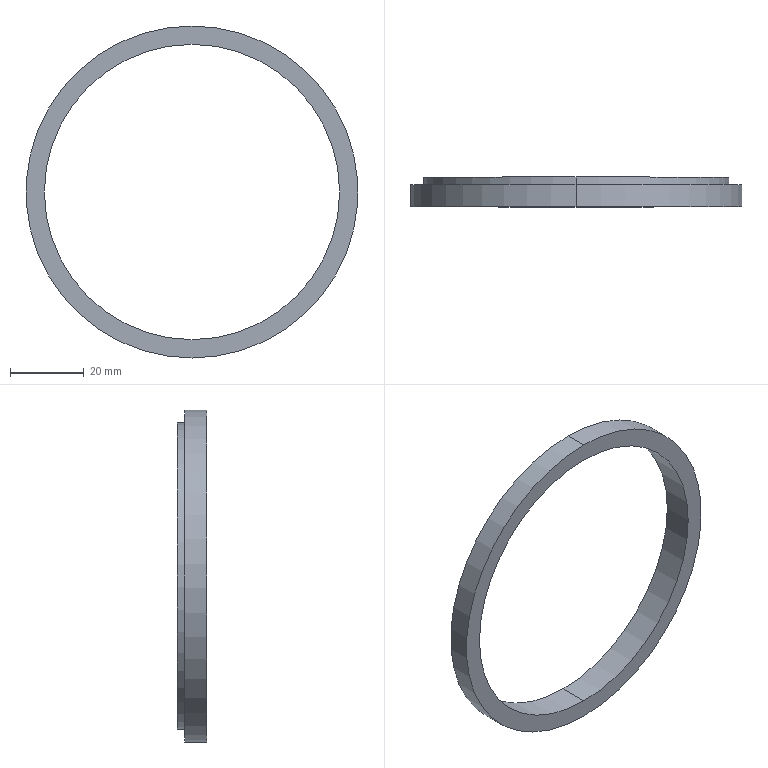Part | SolidWorks | features Extrusion 1, ICE 1 | 1 solid | 9 faces | box 90 x 8 x 90 mm | volume 8779 mm3 | cylinder 6 | plane 3 | commonest cylinder face diameters 80 x2 83 x2 90 x2
STEP:
#1=CARTESIAN_POINT('',(0.,8.,41.5));
#2=VERTEX_POINT('',#1);
#3=CARTESIAN_POINT('',(0.,8.,-41.5));
#4=VERTEX_POINT('',#3);
#5=CARTESIAN_POINT('',(0.,8.,0.));
#6=DIRECTION('',(0.,1.,0.));
#7=DIRECTION('',(0.,0.,1.));
#8=AXIS2_PLACEMENT_3D('',#5,#6,#7);
#9=CIRCLE('',#8,41.5);
#10=EDGE_CURVE('',#2,#4,#9,.T.);
#11=ORIENTED_EDGE('',*,*,#10,.F.);
#12=CARTESIAN_POINT('',(0.,6.,41.5));
#13=VERTEX_POINT('',#12);
#14=CARTESIAN_POINT('',(0.,8.,41.5));
#15=DIRECTION('',(0.,-1.,0.));
#16=VECTOR('',#15,1000.);
#17=LINE('',#14,#16);
#18=EDGE_CURVE('',#2,#13,#17,.T.);
#19=ORIENTED_EDGE('',*,*,#18,.T.);
#20=CARTESIAN_POINT('',(0.,6.,-41.5));
#21=VERTEX_POINT('',#20);
#22=CARTESIAN_POINT('',(0.,6.,0.));
#23=DIRECTION('',(0.,1.,0.));
#24=DIRECTION('',(0.,0.,1.));
#25=AXIS2_PLACEMENT_3D('',#22,#23,#24);
#26=CIRCLE('',#25,41.5);
#27=EDGE_CURVE('',#13,#21,#26,.T.);
#28=ORIENTED_EDGE('',*,*,#27,.T.);
#29=CARTESIAN_POINT('',(0.,8.,-41.5));
#30=DIRECTION('',(0.,-1.,0.));
#31=VECTOR('',#30,1000.);
#32=LINE('',#29,#31);
#33=EDGE_CURVE('',#4,#21,#32,.T.);
#34=ORIENTED_EDGE('',*,*,#33,.F.);
#35=EDGE_LOOP('',(#11,#19,#28,#34));
#36=FACE_OUTER_BOUND('',#35,.T.);
#37=CARTESIAN_POINT('',(0.,8.,0.));
#38=DIRECTION('',(0.,-1.,0.));
#39=DIRECTION('',(0.,0.,-1.));
#40=AXIS2_PLACEMENT_3D('',#37,#38,#39);
#41=CYLINDRICAL_SURFACE('',#40,41.5);
#42=ADVANCED_FACE('',(#36),#41,.T.);
#43=CARTESIAN_POINT('',(0.,8.,-40.));
#44=VERTEX_POINT('',#43);
#45=CARTESIAN_POINT('',(0.,8.,40.));
#46=VERTEX_POINT('',#45);
#47=CARTESIAN_POINT('',(0.,8.,0.));
#48=DIRECTION('',(0.,1.,0.));
#49=DIRECTION('',(0.,0.,1.));
#50=AXIS2_PLACEMENT_3D('',#47,#48,#49);
#51=CIRCLE('',#50,40.);
#52=EDGE_CURVE('',#44,#46,#51,.T.);
#53=ORIENTED_EDGE('',*,*,#52,.T.);
#54=CARTESIAN_POINT('',(0.,0.,40.));
#55=VERTEX_POINT('',#54);
#56=CARTESIAN_POINT('',(0.,6.,40.));
#57=DIRECTION('',(0.,-1.,0.));
#58=VECTOR('',#57,1000.);
#59=LINE('',#56,#58);
#60=EDGE_CURVE('',#46,#55,#59,.T.);
#61=ORIENTED_EDGE('',*,*,#60,.T.);
#62=CARTESIAN_POINT('',(0.,0.,-40.));
#63=VERTEX_POINT('',#62);
#64=CARTESIAN_POINT('',(0.,0.,0.));
#65=DIRECTION('',(0.,1.,0.));
#66=DIRECTION('',(0.,0.,1.));
#67=AXIS2_PLACEMENT_3D('',#64,#65,#66);
#68=CIRCLE('',#67,40.);
#69=EDGE_CURVE('',#63,#55,#68,.T.);
#70=ORIENTED_EDGE('',*,*,#69,.F.);
#71=CARTESIAN_POINT('',(0.,6.,-40.));
#72=DIRECTION('',(0.,-1.,0.));
#73=VECTOR('',#72,1000.);
#74=LINE('',#71,#73);
#75=EDGE_CURVE('',#44,#63,#74,.T.);
#76=ORIENTED_EDGE('',*,*,#75,.F.);
#77=EDGE_LOOP('',(#53,#61,#70,#76));
#78=FACE_OUTER_BOUND('',#77,.T.);
#79=CARTESIAN_POINT('',(0.,6.,0.));
#80=DIRECTION('',(0.,-1.,0.));
#81=DIRECTION('',(0.,0.,-1.));
#82=AXIS2_PLACEMENT_3D('',#79,#80,#81);
#83=CYLINDRICAL_SURFACE('',#82,40.);
#84=ADVANCED_FACE('',(#78),#83,.F.);
#85=CARTESIAN_POINT('',(0.,6.,45.));
#86=VERTEX_POINT('',#85);
#87=CARTESIAN_POINT('',(0.,6.,-45.));
#88=VERTEX_POINT('',#87);
#89=CARTESIAN_POINT('',(0.,6.,0.));
#90=DIRECTION('',(0.,1.,0.));
#91=DIRECTION('',(0.,0.,1.));
#92=AXIS2_PLACEMENT_3D('',#89,#90,#91);
#93=CIRCLE('',#92,45.);
#94=EDGE_CURVE('',#86,#88,#93,.T.);
#95=ORIENTED_EDGE('',*,*,#94,.F.);
#96=CARTESIAN_POINT('',(0.,0.,45.));
#97=VERTEX_POINT('',#96);
#98=CARTESIAN_POINT('',(0.,6.,45.));
#99=DIRECTION('',(0.,-1.,0.));
#100=VECTOR('',#99,1000.);
#101=LINE('',#98,#100);
#102=EDGE_CURVE('',#86,#97,#101,.T.);
#103=ORIENTED_EDGE('',*,*,#102,.T.);
#104=CARTESIAN_POINT('',(0.,0.,-45.));
#105=VERTEX_POINT('',#104);
#106=CARTESIAN_POINT('',(0.,0.,0.));
#107=DIRECTION('',(0.,1.,0.));
#108=DIRECTION('',(0.,0.,1.));
#109=AXIS2_PLACEMENT_3D('',#106,#107,#108);
#110=CIRCLE('',#109,45.);
#111=EDGE_CURVE('',#97,#105,#110,.T.);
#112=ORIENTED_EDGE('',*,*,#111,.T.);
#113=CARTESIAN_POINT('',(0.,6.,-45.));
#114=DIRECTION('',(0.,-1.,0.));
#115=VECTOR('',#114,1000.);
#116=LINE('',#113,#115);
#117=EDGE_CURVE('',#88,#105,#116,.T.);
#118=ORIENTED_EDGE('',*,*,#117,.F.);
#119=EDGE_LOOP('',(#95,#103,#112,#118));
#120=FACE_OUTER_BOUND('',#119,.T.);
#121=CARTESIAN_POINT('',(0.,6.,0.));
#122=DIRECTION('',(0.,-1.,0.));
#123=DIRECTION('',(0.,0.,-1.));
#124=AXIS2_PLACEMENT_3D('',#121,#122,#123);
#125=CYLINDRICAL_SURFACE('',#124,45.);
#126=ADVANCED_FACE('',(#120),#125,.T.);
#127=CARTESIAN_POINT('',(0.,6.,0.));
#128=DIRECTION('',(0.,1.,0.));
#129=DIRECTION('',(0.,0.,1.));
#130=AXIS2_PLACEMENT_3D('',#127,#128,#129);
#131=CIRCLE('',#130,45.);
#132=EDGE_CURVE('',#88,#86,#131,.T.);
#133=ORIENTED_EDGE('',*,*,#132,.T.);
#134=ORIENTED_EDGE('',*,*,#94,.T.);
#135=EDGE_LOOP('',(#133,#134));
#136=FACE_OUTER_BOUND('',#135,.T.);
#137=CARTESIAN_POINT('',(0.,6.,0.));
#138=DIRECTION('',(0.,1.,0.));
#139=DIRECTION('',(0.,0.,1.));
#140=AXIS2_PLACEMENT_3D('',#137,#138,#139);
#141=CIRCLE('',#140,41.5);
#142=EDGE_CURVE('',#21,#13,#141,.T.);
#143=ORIENTED_EDGE('',*,*,#142,.F.);
#144=ORIENTED_EDGE('',*,*,#27,.F.);
#145=EDGE_LOOP('',(#143,#144));
#146=FACE_BOUND('',#145,.T.);
#147=CARTESIAN_POINT('',(0.,6.,0.));
#148=DIRECTION('',(0.,1.,0.));
#149=DIRECTION('',(0.,0.,1.));
#150=AXIS2_PLACEMENT_3D('',#147,#148,#149);
#151=PLANE('',#150);
#152=ADVANCED_FACE('',(#136,#146),#151,.T.);
#153=CARTESIAN_POINT('',(0.,0.,0.));
#154=DIRECTION('',(0.,1.,0.));
#155=DIRECTION('',(0.,0.,1.));
#156=AXIS2_PLACEMENT_3D('',#153,#154,#155);
#157=CIRCLE('',#156,45.);
#158=EDGE_CURVE('',#105,#97,#157,.T.);
#159=ORIENTED_EDGE('',*,*,#158,.F.);
#160=ORIENTED_EDGE('',*,*,#111,.F.);
#161=EDGE_LOOP('',(#159,#160));
#162=FACE_OUTER_BOUND('',#161,.T.);
#163=ORIENTED_EDGE('',*,*,#69,.T.);
#164=CARTESIAN_POINT('',(0.,0.,0.));
#165=DIRECTION('',(0.,1.,0.));
#166=DIRECTION('',(0.,0.,1.));
#167=AXIS2_PLACEMENT_3D('',#164,#165,#166);
#168=CIRCLE('',#167,40.);
#169=EDGE_CURVE('',#55,#63,#168,.T.);
#170=ORIENTED_EDGE('',*,*,#169,.T.);
#171=EDGE_LOOP('',(#163,#170));
#172=FACE_BOUND('',#171,.T.);
#173=CARTESIAN_POINT('',(0.,0.,0.));
#174=DIRECTION('',(0.,1.,0.));
#175=DIRECTION('',(0.,0.,1.));
#176=AXIS2_PLACEMENT_3D('',#173,#174,#175);
#177=PLANE('',#176);
#178=ADVANCED_FACE('',(#162,#172),#177,.F.);
#179=ORIENTED_EDGE('',*,*,#102,.F.);
#180=ORIENTED_EDGE('',*,*,#132,.F.);
#181=ORIENTED_EDGE('',*,*,#117,.T.);
#182=ORIENTED_EDGE('',*,*,#158,.T.);
#183=EDGE_LOOP('',(#179,#180,#181,#182));
#184=FACE_OUTER_BOUND('',#183,.T.);
#185=CARTESIAN_POINT('',(0.,6.,0.));
#186=DIRECTION('',(0.,-1.,0.));
#187=DIRECTION('',(0.,0.,-1.));
#188=AXIS2_PLACEMENT_3D('',#185,#186,#187);
#189=CYLINDRICAL_SURFACE('',#188,45.);
#190=ADVANCED_FACE('',(#184),#189,.T.);
#191=ORIENTED_EDGE('',*,*,#60,.F.);
#192=CARTESIAN_POINT('',(0.,8.,0.));
#193=DIRECTION('',(0.,1.,0.));
#194=DIRECTION('',(0.,0.,1.));
#195=AXIS2_PLACEMENT_3D('',#192,#193,#194);
#196=CIRCLE('',#195,40.);
#197=EDGE_CURVE('',#46,#44,#196,.T.);
#198=ORIENTED_EDGE('',*,*,#197,.T.);
#199=ORIENTED_EDGE('',*,*,#75,.T.);
#200=ORIENTED_EDGE('',*,*,#169,.F.);
#201=EDGE_LOOP('',(#191,#198,#199,#200));
#202=FACE_OUTER_BOUND('',#201,.T.);
#203=CARTESIAN_POINT('',(0.,6.,0.));
#204=DIRECTION('',(0.,-1.,0.));
#205=DIRECTION('',(0.,0.,-1.));
#206=AXIS2_PLACEMENT_3D('',#203,#204,#205);
#207=CYLINDRICAL_SURFACE('',#206,40.);
#208=ADVANCED_FACE('',(#202),#207,.F.);
#209=CARTESIAN_POINT('',(0.,8.,0.));
#210=DIRECTION('',(0.,1.,0.));
#211=DIRECTION('',(0.,0.,1.));
#212=AXIS2_PLACEMENT_3D('',#209,#210,#211);
#213=CIRCLE('',#212,41.5);
#214=EDGE_CURVE('',#4,#2,#213,.T.);
#215=ORIENTED_EDGE('',*,*,#214,.T.);
#216=ORIENTED_EDGE('',*,*,#10,.T.);
#217=EDGE_LOOP('',(#215,#216));
#218=FACE_OUTER_BOUND('',#217,.T.);
#219=ORIENTED_EDGE('',*,*,#52,.F.);
#220=ORIENTED_EDGE('',*,*,#197,.F.);
#221=EDGE_LOOP('',(#219,#220));
#222=FACE_BOUND('',#221,.T.);
#223=CARTESIAN_POINT('',(0.,8.,0.));
#224=DIRECTION('',(0.,1.,0.));
#225=DIRECTION('',(0.,0.,1.));
#226=AXIS2_PLACEMENT_3D('',#223,#224,#225);
#227=PLANE('',#226);
#228=ADVANCED_FACE('',(#218,#222),#227,.T.);
#229=ORIENTED_EDGE('',*,*,#18,.F.);
#230=ORIENTED_EDGE('',*,*,#214,.F.);
#231=ORIENTED_EDGE('',*,*,#33,.T.);
#232=ORIENTED_EDGE('',*,*,#142,.T.);
#233=EDGE_LOOP('',(#229,#230,#231,#232));
#234=FACE_OUTER_BOUND('',#233,.T.);
#235=CARTESIAN_POINT('',(0.,8.,0.));
#236=DIRECTION('',(0.,-1.,0.));
#237=DIRECTION('',(0.,0.,-1.));
#238=AXIS2_PLACEMENT_3D('',#235,#236,#237);
#239=CYLINDRICAL_SURFACE('',#238,41.5);
#240=ADVANCED_FACE('',(#234),#239,.T.);
#241=CLOSED_SHELL('',(#42,#84,#126,#152,#178,#190,#208,#228,#240));
#242=MANIFOLD_SOLID_BREP('',#241);
#243=CARTESIAN_POINT('',(0.,0.,0.));
#244=DIRECTION('',(0.,0.,1.));
#245=DIRECTION('',(1.,0.,0.));
#246=AXIS2_PLACEMENT_3D('',#243,#244,#245);
#247=(LENGTH_UNIT()NAMED_UNIT(*)SI_UNIT(.MILLI.,.METRE.));
#248=UNCERTAINTY_MEASURE_WITH_UNIT(LENGTH_MEASURE(0.00001),#247,'','');
#249=(NAMED_UNIT(*)PLANE_ANGLE_UNIT()SI_UNIT($,.RADIAN.));
#250=(NAMED_UNIT(*)SI_UNIT($,.STERADIAN.)SOLID_ANGLE_UNIT());
#251=(GEOMETRIC_REPRESENTATION_CONTEXT(3)GLOBAL_UNCERTAINTY_ASSIGNED_CONTEXT((#248))GLOBAL_UNIT_ASSIGNED_CONTEXT((#247,#249,#250))REPRESENTATION_CONTEXT('',''));
#252=ADVANCED_BREP_SHAPE_REPRESENTATION('',(#242,#246),#251);